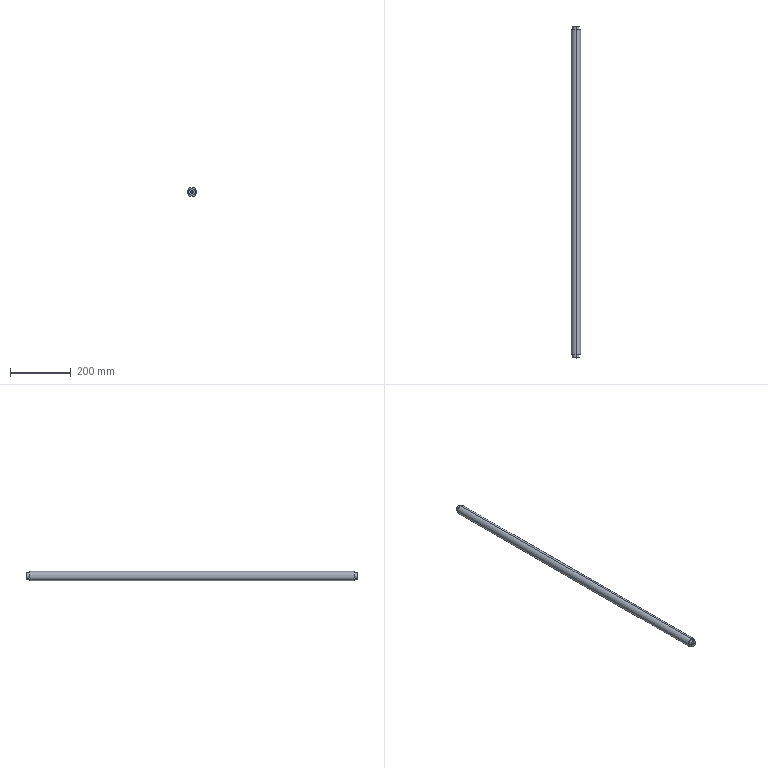Part | SolidWorks | features HoleWzd 2, ICE 2, Extrusion 1 | 1 solid | 18 faces | box 30 x 1095 x 30 mm | volume 765991 mm3 | cylinder 10 | cone 4 | plane 4 | commonest cylinder face diameters 6.8 x4 22 x4 30 x2
STEP:
#1=CARTESIAN_POINT('',(0.,1065.25,-3.4));
#2=VERTEX_POINT('',#1);
#3=CARTESIAN_POINT('',(0.,1065.25,3.4));
#4=VERTEX_POINT('',#3);
#5=CARTESIAN_POINT('',(0.,1065.25,0.));
#6=DIRECTION('',(0.,1.,0.));
#7=DIRECTION('',(0.,0.,1.));
#8=AXIS2_PLACEMENT_3D('',#5,#6,#7);
#9=CIRCLE('',#8,3.4);
#10=EDGE_CURVE('',#2,#4,#9,.T.);
#11=ORIENTED_EDGE('',*,*,#10,.F.);
#12=CARTESIAN_POINT('',(0.,1085.,-3.4));
#13=VERTEX_POINT('',#12);
#14=CARTESIAN_POINT('',(0.,1085.,-3.4));
#15=DIRECTION('',(0.,1.,0.));
#16=VECTOR('',#15,1000.);
#17=LINE('',#14,#16);
#18=EDGE_CURVE('',#2,#13,#17,.T.);
#19=ORIENTED_EDGE('',*,*,#18,.T.);
#20=CARTESIAN_POINT('',(0.,1085.,3.4));
#21=VERTEX_POINT('',#20);
#22=CARTESIAN_POINT('',(0.,1085.,0.));
#23=DIRECTION('',(0.,1.,0.));
#24=DIRECTION('',(0.,0.,1.));
#25=AXIS2_PLACEMENT_3D('',#22,#23,#24);
#26=CIRCLE('',#25,3.4);
#27=EDGE_CURVE('',#13,#21,#26,.T.);
#28=ORIENTED_EDGE('',*,*,#27,.T.);
#29=CARTESIAN_POINT('',(0.,1085.,3.4));
#30=DIRECTION('',(0.,1.,0.));
#31=VECTOR('',#30,1000.);
#32=LINE('',#29,#31);
#33=EDGE_CURVE('',#4,#21,#32,.T.);
#34=ORIENTED_EDGE('',*,*,#33,.F.);
#35=EDGE_LOOP('',(#11,#19,#28,#34));
#36=FACE_OUTER_BOUND('',#35,.T.);
#37=CARTESIAN_POINT('',(0.,1085.,0.));
#38=DIRECTION('',(0.,1.,0.));
#39=DIRECTION('',(0.,0.,1.));
#40=AXIS2_PLACEMENT_3D('',#37,#38,#39);
#41=CYLINDRICAL_SURFACE('',#40,3.4);
#42=ADVANCED_FACE('',(#36),#41,.F.);
#43=CARTESIAN_POINT('',(0.,1063.207,0.));
#44=VERTEX_POINT('',#43);
#45=CARTESIAN_POINT('',(0.,1065.25,3.4));
#46=DIRECTION('',(0.,0.515,0.8572));
#47=VECTOR('',#46,1000.);
#48=LINE('',#45,#47);
#49=EDGE_CURVE('',#44,#4,#48,.T.);
#50=ORIENTED_EDGE('',*,*,#49,.F.);
#51=CARTESIAN_POINT('',(0.,1065.25,-3.4));
#52=DIRECTION('',(0.,0.515,-0.8572));
#53=VECTOR('',#52,1000.);
#54=LINE('',#51,#53);
#55=EDGE_CURVE('',#44,#2,#54,.T.);
#56=ORIENTED_EDGE('',*,*,#55,.T.);
#57=ORIENTED_EDGE('',*,*,#10,.T.);
#58=EDGE_LOOP('',(#50,#56,#57));
#59=FACE_OUTER_BOUND('',#58,.T.);
#60=CARTESIAN_POINT('',(0.,1065.25,0.));
#61=DIRECTION('',(0.,1.,0.));
#62=DIRECTION('',(0.,0.,1.));
#63=AXIS2_PLACEMENT_3D('',#60,#61,#62);
#64=CONICAL_SURFACE('',#63,3.4,1.03);
#65=ADVANCED_FACE('',(#59),#64,.F.);
#66=CARTESIAN_POINT('',(0.,9.75,3.4));
#67=VERTEX_POINT('',#66);
#68=CARTESIAN_POINT('',(0.,9.75,-3.4));
#69=VERTEX_POINT('',#68);
#70=CARTESIAN_POINT('',(0.,9.75,0.));
#71=DIRECTION('',(0.,-1.,0.));
#72=DIRECTION('',(0.,0.,-1.));
#73=AXIS2_PLACEMENT_3D('',#70,#71,#72);
#74=CIRCLE('',#73,3.4);
#75=EDGE_CURVE('',#67,#69,#74,.T.);
#76=ORIENTED_EDGE('',*,*,#75,.F.);
#77=CARTESIAN_POINT('',(0.,-10.,3.4));
#78=VERTEX_POINT('',#77);
#79=CARTESIAN_POINT('',(0.,-10.,3.4));
#80=DIRECTION('',(0.,-1.,0.));
#81=VECTOR('',#80,1000.);
#82=LINE('',#79,#81);
#83=EDGE_CURVE('',#67,#78,#82,.T.);
#84=ORIENTED_EDGE('',*,*,#83,.T.);
#85=CARTESIAN_POINT('',(0.,-10.,-3.4));
#86=VERTEX_POINT('',#85);
#87=CARTESIAN_POINT('',(0.,-10.,0.));
#88=DIRECTION('',(0.,-1.,0.));
#89=DIRECTION('',(0.,0.,-1.));
#90=AXIS2_PLACEMENT_3D('',#87,#88,#89);
#91=CIRCLE('',#90,3.4);
#92=EDGE_CURVE('',#78,#86,#91,.T.);
#93=ORIENTED_EDGE('',*,*,#92,.T.);
#94=CARTESIAN_POINT('',(0.,-10.,-3.4));
#95=DIRECTION('',(0.,-1.,0.));
#96=VECTOR('',#95,1000.);
#97=LINE('',#94,#96);
#98=EDGE_CURVE('',#69,#86,#97,.T.);
#99=ORIENTED_EDGE('',*,*,#98,.F.);
#100=EDGE_LOOP('',(#76,#84,#93,#99));
#101=FACE_OUTER_BOUND('',#100,.T.);
#102=CARTESIAN_POINT('',(0.,-10.,0.));
#103=DIRECTION('',(0.,-1.,0.));
#104=DIRECTION('',(0.,0.,-1.));
#105=AXIS2_PLACEMENT_3D('',#102,#103,#104);
#106=CYLINDRICAL_SURFACE('',#105,3.4);
#107=ADVANCED_FACE('',(#101),#106,.F.);
#108=CARTESIAN_POINT('',(0.,11.793,0.));
#109=VERTEX_POINT('',#108);
#110=CARTESIAN_POINT('',(0.,9.75,-3.4));
#111=DIRECTION('',(0.,-0.515,-0.8572));
#112=VECTOR('',#111,1000.);
#113=LINE('',#110,#112);
#114=EDGE_CURVE('',#109,#69,#113,.T.);
#115=ORIENTED_EDGE('',*,*,#114,.F.);
#116=CARTESIAN_POINT('',(0.,9.75,3.4));
#117=DIRECTION('',(0.,-0.515,0.8572));
#118=VECTOR('',#117,1000.);
#119=LINE('',#116,#118);
#120=EDGE_CURVE('',#109,#67,#119,.T.);
#121=ORIENTED_EDGE('',*,*,#120,.T.);
#122=ORIENTED_EDGE('',*,*,#75,.T.);
#123=EDGE_LOOP('',(#115,#121,#122));
#124=FACE_OUTER_BOUND('',#123,.T.);
#125=CARTESIAN_POINT('',(0.,9.75,0.));
#126=DIRECTION('',(0.,-1.,0.));
#127=DIRECTION('',(0.,0.,-1.));
#128=AXIS2_PLACEMENT_3D('',#125,#126,#127);
#129=CONICAL_SURFACE('',#128,3.4,1.03);
#130=ADVANCED_FACE('',(#124),#129,.F.);
#131=CARTESIAN_POINT('',(0.,-10.,-11.));
#132=VERTEX_POINT('',#131);
#133=CARTESIAN_POINT('',(0.,-10.,11.));
#134=VERTEX_POINT('',#133);
#135=CARTESIAN_POINT('',(0.,-10.,0.));
#136=DIRECTION('',(0.,-1.,0.));
#137=DIRECTION('',(0.,0.,-1.));
#138=AXIS2_PLACEMENT_3D('',#135,#136,#137);
#139=CIRCLE('',#138,11.);
#140=EDGE_CURVE('',#132,#134,#139,.T.);
#141=ORIENTED_EDGE('',*,*,#140,.F.);
#142=CARTESIAN_POINT('',(0.,0.,-11.));
#143=VERTEX_POINT('',#142);
#144=CARTESIAN_POINT('',(0.,-10.,-11.));
#145=DIRECTION('',(0.,1.,0.));
#146=VECTOR('',#145,1000.);
#147=LINE('',#144,#146);
#148=EDGE_CURVE('',#132,#143,#147,.T.);
#149=ORIENTED_EDGE('',*,*,#148,.T.);
#150=CARTESIAN_POINT('',(0.,0.,11.));
#151=VERTEX_POINT('',#150);
#152=CARTESIAN_POINT('',(0.,0.,0.));
#153=DIRECTION('',(0.,-1.,0.));
#154=DIRECTION('',(0.,0.,-1.));
#155=AXIS2_PLACEMENT_3D('',#152,#153,#154);
#156=CIRCLE('',#155,11.);
#157=EDGE_CURVE('',#143,#151,#156,.T.);
#158=ORIENTED_EDGE('',*,*,#157,.T.);
#159=CARTESIAN_POINT('',(0.,-10.,11.));
#160=DIRECTION('',(0.,1.,0.));
#161=VECTOR('',#160,1000.);
#162=LINE('',#159,#161);
#163=EDGE_CURVE('',#134,#151,#162,.T.);
#164=ORIENTED_EDGE('',*,*,#163,.F.);
#165=EDGE_LOOP('',(#141,#149,#158,#164));
#166=FACE_OUTER_BOUND('',#165,.T.);
#167=CARTESIAN_POINT('',(0.,-10.,0.));
#168=DIRECTION('',(0.,1.,0.));
#169=DIRECTION('',(0.,0.,1.));
#170=AXIS2_PLACEMENT_3D('',#167,#168,#169);
#171=CYLINDRICAL_SURFACE('',#170,11.);
#172=ADVANCED_FACE('',(#166),#171,.T.);
#173=CARTESIAN_POINT('',(0.,1085.,11.));
#174=VERTEX_POINT('',#173);
#175=CARTESIAN_POINT('',(0.,1085.,-11.));
#176=VERTEX_POINT('',#175);
#177=CARTESIAN_POINT('',(0.,1085.,0.));
#178=DIRECTION('',(0.,1.,0.));
#179=DIRECTION('',(0.,0.,1.));
#180=AXIS2_PLACEMENT_3D('',#177,#178,#179);
#181=CIRCLE('',#180,11.);
#182=EDGE_CURVE('',#174,#176,#181,.T.);
#183=ORIENTED_EDGE('',*,*,#182,.F.);
#184=CARTESIAN_POINT('',(0.,1075.,11.));
#185=VERTEX_POINT('',#184);
#186=CARTESIAN_POINT('',(0.,1085.,11.));
#187=DIRECTION('',(0.,-1.,0.));
#188=VECTOR('',#187,1000.);
#189=LINE('',#186,#188);
#190=EDGE_CURVE('',#174,#185,#189,.T.);
#191=ORIENTED_EDGE('',*,*,#190,.T.);
#192=CARTESIAN_POINT('',(0.,1075.,-11.));
#193=VERTEX_POINT('',#192);
#194=CARTESIAN_POINT('',(0.,1075.,0.));
#195=DIRECTION('',(0.,1.,0.));
#196=DIRECTION('',(0.,0.,1.));
#197=AXIS2_PLACEMENT_3D('',#194,#195,#196);
#198=CIRCLE('',#197,11.);
#199=EDGE_CURVE('',#185,#193,#198,.T.);
#200=ORIENTED_EDGE('',*,*,#199,.T.);
#201=CARTESIAN_POINT('',(0.,1085.,-11.));
#202=DIRECTION('',(0.,-1.,0.));
#203=VECTOR('',#202,1000.);
#204=LINE('',#201,#203);
#205=EDGE_CURVE('',#176,#193,#204,.T.);
#206=ORIENTED_EDGE('',*,*,#205,.F.);
#207=EDGE_LOOP('',(#183,#191,#200,#206));
#208=FACE_OUTER_BOUND('',#207,.T.);
#209=CARTESIAN_POINT('',(0.,1085.,0.));
#210=DIRECTION('',(0.,-1.,0.));
#211=DIRECTION('',(0.,0.,-1.));
#212=AXIS2_PLACEMENT_3D('',#209,#210,#211);
#213=CYLINDRICAL_SURFACE('',#212,11.);
#214=ADVANCED_FACE('',(#208),#213,.T.);
#215=CARTESIAN_POINT('',(0.,1075.,15.));
#216=VERTEX_POINT('',#215);
#217=CARTESIAN_POINT('',(0.,1075.,-15.));
#218=VERTEX_POINT('',#217);
#219=CARTESIAN_POINT('',(0.,1075.,0.));
#220=DIRECTION('',(0.,1.,0.));
#221=DIRECTION('',(0.,0.,1.));
#222=AXIS2_PLACEMENT_3D('',#219,#220,#221);
#223=CIRCLE('',#222,15.);
#224=EDGE_CURVE('',#216,#218,#223,.T.);
#225=ORIENTED_EDGE('',*,*,#224,.F.);
#226=CARTESIAN_POINT('',(0.,0.,15.));
#227=VERTEX_POINT('',#226);
#228=CARTESIAN_POINT('',(0.,1075.,15.));
#229=DIRECTION('',(0.,-1.,0.));
#230=VECTOR('',#229,1000.);
#231=LINE('',#228,#230);
#232=EDGE_CURVE('',#216,#227,#231,.T.);
#233=ORIENTED_EDGE('',*,*,#232,.T.);
#234=CARTESIAN_POINT('',(0.,0.,-15.));
#235=VERTEX_POINT('',#234);
#236=CARTESIAN_POINT('',(0.,0.,0.));
#237=DIRECTION('',(0.,1.,0.));
#238=DIRECTION('',(0.,0.,1.));
#239=AXIS2_PLACEMENT_3D('',#236,#237,#238);
#240=CIRCLE('',#239,15.);
#241=EDGE_CURVE('',#227,#235,#240,.T.);
#242=ORIENTED_EDGE('',*,*,#241,.T.);
#243=CARTESIAN_POINT('',(0.,1075.,-15.));
#244=DIRECTION('',(0.,-1.,0.));
#245=VECTOR('',#244,1000.);
#246=LINE('',#243,#245);
#247=EDGE_CURVE('',#218,#235,#246,.T.);
#248=ORIENTED_EDGE('',*,*,#247,.F.);
#249=EDGE_LOOP('',(#225,#233,#242,#248));
#250=FACE_OUTER_BOUND('',#249,.T.);
#251=CARTESIAN_POINT('',(0.,1075.,0.));
#252=DIRECTION('',(0.,-1.,0.));
#253=DIRECTION('',(0.,0.,-1.));
#254=AXIS2_PLACEMENT_3D('',#251,#252,#253);
#255=CYLINDRICAL_SURFACE('',#254,15.);
#256=ADVANCED_FACE('',(#250),#255,.T.);
#257=ORIENTED_EDGE('',*,*,#232,.F.);
#258=CARTESIAN_POINT('',(0.,1075.,0.));
#259=DIRECTION('',(0.,1.,0.));
#260=DIRECTION('',(0.,0.,1.));
#261=AXIS2_PLACEMENT_3D('',#258,#259,#260);
#262=CIRCLE('',#261,15.);
#263=EDGE_CURVE('',#218,#216,#262,.T.);
#264=ORIENTED_EDGE('',*,*,#263,.F.);
#265=ORIENTED_EDGE('',*,*,#247,.T.);
#266=CARTESIAN_POINT('',(0.,0.,0.));
#267=DIRECTION('',(0.,1.,0.));
#268=DIRECTION('',(0.,0.,1.));
#269=AXIS2_PLACEMENT_3D('',#266,#267,#268);
#270=CIRCLE('',#269,15.);
#271=EDGE_CURVE('',#235,#227,#270,.T.);
#272=ORIENTED_EDGE('',*,*,#271,.T.);
#273=EDGE_LOOP('',(#257,#264,#265,#272));
#274=FACE_OUTER_BOUND('',#273,.T.);
#275=CARTESIAN_POINT('',(0.,1075.,0.));
#276=DIRECTION('',(0.,-1.,0.));
#277=DIRECTION('',(0.,0.,-1.));
#278=AXIS2_PLACEMENT_3D('',#275,#276,#277);
#279=CYLINDRICAL_SURFACE('',#278,15.);
#280=ADVANCED_FACE('',(#274),#279,.T.);
#281=CARTESIAN_POINT('',(0.,1075.,0.));
#282=DIRECTION('',(0.,1.,0.));
#283=DIRECTION('',(0.,0.,1.));
#284=AXIS2_PLACEMENT_3D('',#281,#282,#283);
#285=CIRCLE('',#284,11.);
#286=EDGE_CURVE('',#193,#185,#285,.T.);
#287=ORIENTED_EDGE('',*,*,#286,.F.);
#288=ORIENTED_EDGE('',*,*,#199,.F.);
#289=EDGE_LOOP('',(#287,#288));
#290=FACE_BOUND('',#289,.T.);
#291=ORIENTED_EDGE('',*,*,#263,.T.);
#292=ORIENTED_EDGE('',*,*,#224,.T.);
#293=EDGE_LOOP('',(#291,#292));
#294=FACE_OUTER_BOUND('',#293,.T.);
#295=CARTESIAN_POINT('',(0.,1075.,0.));
#296=DIRECTION('',(0.,1.,0.));
#297=DIRECTION('',(0.,0.,1.));
#298=AXIS2_PLACEMENT_3D('',#295,#296,#297);
#299=PLANE('',#298);
#300=ADVANCED_FACE('',(#290,#294),#299,.T.);
#301=CARTESIAN_POINT('',(0.,0.,0.));
#302=DIRECTION('',(0.,-1.,0.));
#303=DIRECTION('',(0.,0.,-1.));
#304=AXIS2_PLACEMENT_3D('',#301,#302,#303);
#305=CIRCLE('',#304,11.);
#306=EDGE_CURVE('',#151,#143,#305,.T.);
#307=ORIENTED_EDGE('',*,*,#306,.F.);
#308=ORIENTED_EDGE('',*,*,#157,.F.);
#309=EDGE_LOOP('',(#307,#308));
#310=FACE_BOUND('',#309,.T.);
#311=ORIENTED_EDGE('',*,*,#271,.F.);
#312=ORIENTED_EDGE('',*,*,#241,.F.);
#313=EDGE_LOOP('',(#311,#312));
#314=FACE_OUTER_BOUND('',#313,.T.);
#315=CARTESIAN_POINT('',(0.,0.,0.));
#316=DIRECTION('',(0.,1.,0.));
#317=DIRECTION('',(0.,0.,1.));
#318=AXIS2_PLACEMENT_3D('',#315,#316,#317);
#319=PLANE('',#318);
#320=ADVANCED_FACE('',(#310,#314),#319,.F.);
#321=ORIENTED_EDGE('',*,*,#190,.F.);
#322=CARTESIAN_POINT('',(0.,1085.,0.));
#323=DIRECTION('',(0.,1.,0.));
#324=DIRECTION('',(0.,0.,1.));
#325=AXIS2_PLACEMENT_3D('',#322,#323,#324);
#326=CIRCLE('',#325,11.);
#327=EDGE_CURVE('',#176,#174,#326,.T.);
#328=ORIENTED_EDGE('',*,*,#327,.F.);
#329=ORIENTED_EDGE('',*,*,#205,.T.);
#330=ORIENTED_EDGE('',*,*,#286,.T.);
#331=EDGE_LOOP('',(#321,#328,#329,#330));
#332=FACE_OUTER_BOUND('',#331,.T.);
#333=CARTESIAN_POINT('',(0.,1085.,0.));
#334=DIRECTION('',(0.,-1.,0.));
#335=DIRECTION('',(0.,0.,-1.));
#336=AXIS2_PLACEMENT_3D('',#333,#334,#335);
#337=CYLINDRICAL_SURFACE('',#336,11.);
#338=ADVANCED_FACE('',(#332),#337,.T.);
#339=CARTESIAN_POINT('',(0.,1085.,0.));
#340=DIRECTION('',(0.,1.,0.));
#341=DIRECTION('',(0.,0.,1.));
#342=AXIS2_PLACEMENT_3D('',#339,#340,#341);
#343=CIRCLE('',#342,3.4);
#344=EDGE_CURVE('',#21,#13,#343,.T.);
#345=ORIENTED_EDGE('',*,*,#344,.F.);
#346=ORIENTED_EDGE('',*,*,#27,.F.);
#347=EDGE_LOOP('',(#345,#346));
#348=FACE_BOUND('',#347,.T.);
#349=ORIENTED_EDGE('',*,*,#327,.T.);
#350=ORIENTED_EDGE('',*,*,#182,.T.);
#351=EDGE_LOOP('',(#349,#350));
#352=FACE_OUTER_BOUND('',#351,.T.);
#353=CARTESIAN_POINT('',(0.,1085.,0.));
#354=DIRECTION('',(0.,1.,0.));
#355=DIRECTION('',(0.,0.,1.));
#356=AXIS2_PLACEMENT_3D('',#353,#354,#355);
#357=PLANE('',#356);
#358=ADVANCED_FACE('',(#348,#352),#357,.T.);
#359=ORIENTED_EDGE('',*,*,#148,.F.);
#360=CARTESIAN_POINT('',(0.,-10.,0.));
#361=DIRECTION('',(0.,-1.,0.));
#362=DIRECTION('',(0.,0.,-1.));
#363=AXIS2_PLACEMENT_3D('',#360,#361,#362);
#364=CIRCLE('',#363,11.);
#365=EDGE_CURVE('',#134,#132,#364,.T.);
#366=ORIENTED_EDGE('',*,*,#365,.F.);
#367=ORIENTED_EDGE('',*,*,#163,.T.);
#368=ORIENTED_EDGE('',*,*,#306,.T.);
#369=EDGE_LOOP('',(#359,#366,#367,#368));
#370=FACE_OUTER_BOUND('',#369,.T.);
#371=CARTESIAN_POINT('',(0.,-10.,0.));
#372=DIRECTION('',(0.,1.,0.));
#373=DIRECTION('',(0.,0.,1.));
#374=AXIS2_PLACEMENT_3D('',#371,#372,#373);
#375=CYLINDRICAL_SURFACE('',#374,11.);
#376=ADVANCED_FACE('',(#370),#375,.T.);
#377=CARTESIAN_POINT('',(0.,-10.,0.));
#378=DIRECTION('',(0.,-1.,0.));
#379=DIRECTION('',(0.,0.,-1.));
#380=AXIS2_PLACEMENT_3D('',#377,#378,#379);
#381=CIRCLE('',#380,3.4);
#382=EDGE_CURVE('',#86,#78,#381,.T.);
#383=ORIENTED_EDGE('',*,*,#382,.F.);
#384=ORIENTED_EDGE('',*,*,#92,.F.);
#385=EDGE_LOOP('',(#383,#384));
#386=FACE_BOUND('',#385,.T.);
#387=ORIENTED_EDGE('',*,*,#365,.T.);
#388=ORIENTED_EDGE('',*,*,#140,.T.);
#389=EDGE_LOOP('',(#387,#388));
#390=FACE_OUTER_BOUND('',#389,.T.);
#391=CARTESIAN_POINT('',(0.,-10.,0.));
#392=DIRECTION('',(0.,-1.,0.));
#393=DIRECTION('',(0.,0.,-1.));
#394=AXIS2_PLACEMENT_3D('',#391,#392,#393);
#395=PLANE('',#394);
#396=ADVANCED_FACE('',(#386,#390),#395,.T.);
#397=ORIENTED_EDGE('',*,*,#120,.F.);
#398=ORIENTED_EDGE('',*,*,#114,.T.);
#399=CARTESIAN_POINT('',(0.,9.75,0.));
#400=DIRECTION('',(0.,-1.,0.));
#401=DIRECTION('',(0.,0.,-1.));
#402=AXIS2_PLACEMENT_3D('',#399,#400,#401);
#403=CIRCLE('',#402,3.4);
#404=EDGE_CURVE('',#69,#67,#403,.T.);
#405=ORIENTED_EDGE('',*,*,#404,.T.);
#406=EDGE_LOOP('',(#397,#398,#405));
#407=FACE_OUTER_BOUND('',#406,.T.);
#408=CARTESIAN_POINT('',(0.,9.75,0.));
#409=DIRECTION('',(0.,-1.,0.));
#410=DIRECTION('',(0.,0.,-1.));
#411=AXIS2_PLACEMENT_3D('',#408,#409,#410);
#412=CONICAL_SURFACE('',#411,3.4,1.03);
#413=ADVANCED_FACE('',(#407),#412,.F.);
#414=ORIENTED_EDGE('',*,*,#83,.F.);
#415=ORIENTED_EDGE('',*,*,#404,.F.);
#416=ORIENTED_EDGE('',*,*,#98,.T.);
#417=ORIENTED_EDGE('',*,*,#382,.T.);
#418=EDGE_LOOP('',(#414,#415,#416,#417));
#419=FACE_OUTER_BOUND('',#418,.T.);
#420=CARTESIAN_POINT('',(0.,-10.,0.));
#421=DIRECTION('',(0.,-1.,0.));
#422=DIRECTION('',(0.,0.,-1.));
#423=AXIS2_PLACEMENT_3D('',#420,#421,#422);
#424=CYLINDRICAL_SURFACE('',#423,3.4);
#425=ADVANCED_FACE('',(#419),#424,.F.);
#426=ORIENTED_EDGE('',*,*,#55,.F.);
#427=ORIENTED_EDGE('',*,*,#49,.T.);
#428=CARTESIAN_POINT('',(0.,1065.25,0.));
#429=DIRECTION('',(0.,1.,0.));
#430=DIRECTION('',(0.,0.,1.));
#431=AXIS2_PLACEMENT_3D('',#428,#429,#430);
#432=CIRCLE('',#431,3.4);
#433=EDGE_CURVE('',#4,#2,#432,.T.);
#434=ORIENTED_EDGE('',*,*,#433,.T.);
#435=EDGE_LOOP('',(#426,#427,#434));
#436=FACE_OUTER_BOUND('',#435,.T.);
#437=CARTESIAN_POINT('',(0.,1065.25,0.));
#438=DIRECTION('',(0.,1.,0.));
#439=DIRECTION('',(0.,0.,1.));
#440=AXIS2_PLACEMENT_3D('',#437,#438,#439);
#441=CONICAL_SURFACE('',#440,3.4,1.03);
#442=ADVANCED_FACE('',(#436),#441,.F.);
#443=ORIENTED_EDGE('',*,*,#18,.F.);
#444=ORIENTED_EDGE('',*,*,#433,.F.);
#445=ORIENTED_EDGE('',*,*,#33,.T.);
#446=ORIENTED_EDGE('',*,*,#344,.T.);
#447=EDGE_LOOP('',(#443,#444,#445,#446));
#448=FACE_OUTER_BOUND('',#447,.T.);
#449=CARTESIAN_POINT('',(0.,1085.,0.));
#450=DIRECTION('',(0.,1.,0.));
#451=DIRECTION('',(0.,0.,1.));
#452=AXIS2_PLACEMENT_3D('',#449,#450,#451);
#453=CYLINDRICAL_SURFACE('',#452,3.4);
#454=ADVANCED_FACE('',(#448),#453,.F.);
#455=CLOSED_SHELL('',(#42,#65,#107,#130,#172,#214,#256,#280,#300,#320,#338,#358,#376,#396,#413,#425,#442,#454));
#456=MANIFOLD_SOLID_BREP('',#455);
#457=CARTESIAN_POINT('',(0.,0.,0.));
#458=DIRECTION('',(0.,0.,1.));
#459=DIRECTION('',(1.,0.,0.));
#460=AXIS2_PLACEMENT_3D('',#457,#458,#459);
#461=(LENGTH_UNIT()NAMED_UNIT(*)SI_UNIT(.MILLI.,.METRE.));
#462=UNCERTAINTY_MEASURE_WITH_UNIT(LENGTH_MEASURE(0.00001),#461,'','');
#463=(NAMED_UNIT(*)PLANE_ANGLE_UNIT()SI_UNIT($,.RADIAN.));
#464=(NAMED_UNIT(*)SI_UNIT($,.STERADIAN.)SOLID_ANGLE_UNIT());
#465=(GEOMETRIC_REPRESENTATION_CONTEXT(3)GLOBAL_UNCERTAINTY_ASSIGNED_CONTEXT((#462))GLOBAL_UNIT_ASSIGNED_CONTEXT((#461,#463,#464))REPRESENTATION_CONTEXT('',''));
#466=ADVANCED_BREP_SHAPE_REPRESENTATION('',(#456,#460),#465);